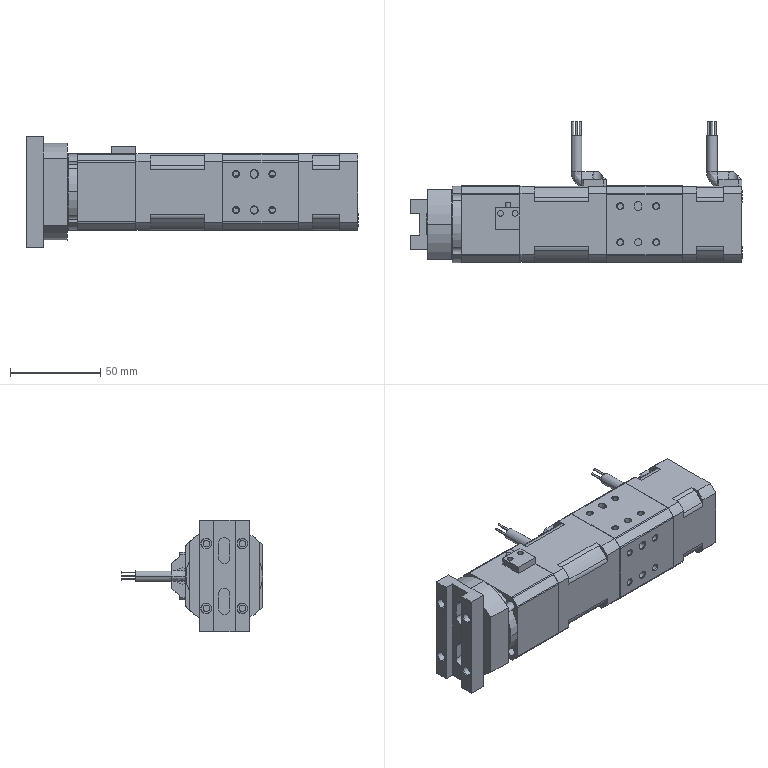Part | SolidWorks | 3 solids | 661 faces | box 184.2 x 78.5 x 62 mm | volume 299098 mm3 | cylinder 305 | plane 274 | cone 74 | spline 8 | commonest cylinder face diameters 3.3 x32 2.5 x30 2 x28 3.2 x28 54 x19 8 x18